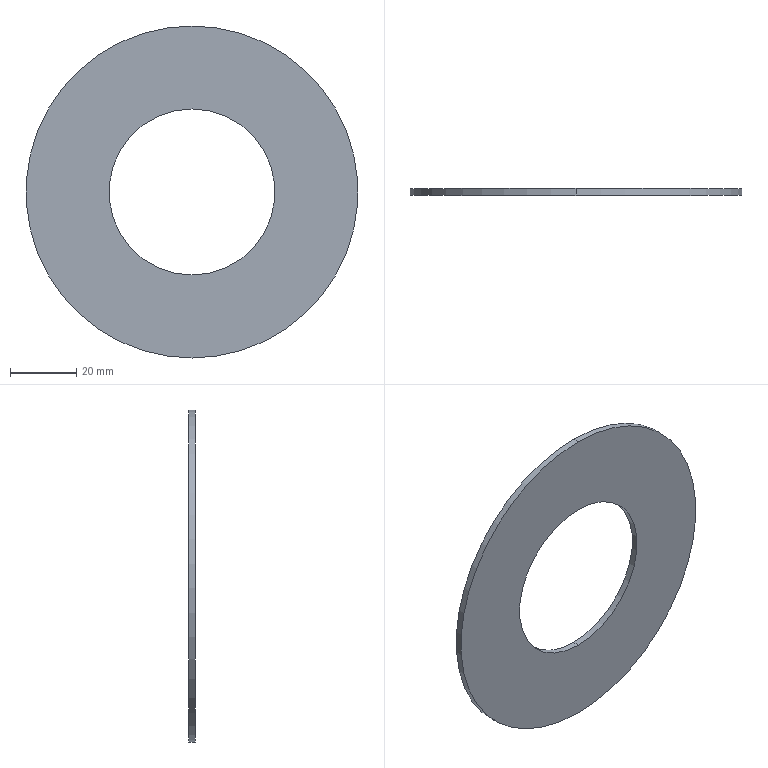Part | SolidWorks | features Extrusion 1 | 1 solid | 6 faces | box 100 x 2 x 100 mm | volume 11781 mm3 | cylinder 4 | plane 2 | commonest cylinder face diameters 50 x2 100 x2
STEP:
#1=CARTESIAN_POINT('',(0.,2.,-25.));
#2=VERTEX_POINT('',#1);
#3=CARTESIAN_POINT('',(0.,2.,25.));
#4=VERTEX_POINT('',#3);
#5=CARTESIAN_POINT('',(0.,2.,0.));
#6=DIRECTION('',(0.,1.,0.));
#7=DIRECTION('',(0.,0.,1.));
#8=AXIS2_PLACEMENT_3D('',#5,#6,#7);
#9=CIRCLE('',#8,25.);
#10=EDGE_CURVE('',#2,#4,#9,.T.);
#11=ORIENTED_EDGE('',*,*,#10,.T.);
#12=CARTESIAN_POINT('',(0.,0.,25.));
#13=VERTEX_POINT('',#12);
#14=CARTESIAN_POINT('',(0.,2.,25.));
#15=DIRECTION('',(0.,-1.,0.));
#16=VECTOR('',#15,1000.);
#17=LINE('',#14,#16);
#18=EDGE_CURVE('',#4,#13,#17,.T.);
#19=ORIENTED_EDGE('',*,*,#18,.T.);
#20=CARTESIAN_POINT('',(0.,0.,-25.));
#21=VERTEX_POINT('',#20);
#22=CARTESIAN_POINT('',(0.,0.,0.));
#23=DIRECTION('',(0.,1.,0.));
#24=DIRECTION('',(0.,0.,1.));
#25=AXIS2_PLACEMENT_3D('',#22,#23,#24);
#26=CIRCLE('',#25,25.);
#27=EDGE_CURVE('',#21,#13,#26,.T.);
#28=ORIENTED_EDGE('',*,*,#27,.F.);
#29=CARTESIAN_POINT('',(0.,2.,-25.));
#30=DIRECTION('',(0.,-1.,0.));
#31=VECTOR('',#30,1000.);
#32=LINE('',#29,#31);
#33=EDGE_CURVE('',#2,#21,#32,.T.);
#34=ORIENTED_EDGE('',*,*,#33,.F.);
#35=EDGE_LOOP('',(#11,#19,#28,#34));
#36=FACE_OUTER_BOUND('',#35,.T.);
#37=CARTESIAN_POINT('',(0.,2.,0.));
#38=DIRECTION('',(0.,-1.,0.));
#39=DIRECTION('',(0.,0.,-1.));
#40=AXIS2_PLACEMENT_3D('',#37,#38,#39);
#41=CYLINDRICAL_SURFACE('',#40,25.);
#42=ADVANCED_FACE('',(#36),#41,.F.);
#43=CARTESIAN_POINT('',(0.,2.,50.));
#44=VERTEX_POINT('',#43);
#45=CARTESIAN_POINT('',(0.,2.,-50.));
#46=VERTEX_POINT('',#45);
#47=CARTESIAN_POINT('',(0.,2.,0.));
#48=DIRECTION('',(0.,1.,0.));
#49=DIRECTION('',(0.,0.,1.));
#50=AXIS2_PLACEMENT_3D('',#47,#48,#49);
#51=CIRCLE('',#50,50.);
#52=EDGE_CURVE('',#44,#46,#51,.T.);
#53=ORIENTED_EDGE('',*,*,#52,.F.);
#54=CARTESIAN_POINT('',(0.,0.,50.));
#55=VERTEX_POINT('',#54);
#56=CARTESIAN_POINT('',(0.,2.,50.));
#57=DIRECTION('',(0.,-1.,0.));
#58=VECTOR('',#57,1000.);
#59=LINE('',#56,#58);
#60=EDGE_CURVE('',#44,#55,#59,.T.);
#61=ORIENTED_EDGE('',*,*,#60,.T.);
#62=CARTESIAN_POINT('',(0.,0.,-50.));
#63=VERTEX_POINT('',#62);
#64=CARTESIAN_POINT('',(0.,0.,0.));
#65=DIRECTION('',(0.,1.,0.));
#66=DIRECTION('',(0.,0.,1.));
#67=AXIS2_PLACEMENT_3D('',#64,#65,#66);
#68=CIRCLE('',#67,50.);
#69=EDGE_CURVE('',#55,#63,#68,.T.);
#70=ORIENTED_EDGE('',*,*,#69,.T.);
#71=CARTESIAN_POINT('',(0.,2.,-50.));
#72=DIRECTION('',(0.,-1.,0.));
#73=VECTOR('',#72,1000.);
#74=LINE('',#71,#73);
#75=EDGE_CURVE('',#46,#63,#74,.T.);
#76=ORIENTED_EDGE('',*,*,#75,.F.);
#77=EDGE_LOOP('',(#53,#61,#70,#76));
#78=FACE_OUTER_BOUND('',#77,.T.);
#79=CARTESIAN_POINT('',(0.,2.,0.));
#80=DIRECTION('',(0.,-1.,0.));
#81=DIRECTION('',(0.,0.,-1.));
#82=AXIS2_PLACEMENT_3D('',#79,#80,#81);
#83=CYLINDRICAL_SURFACE('',#82,50.);
#84=ADVANCED_FACE('',(#78),#83,.T.);
#85=CARTESIAN_POINT('',(0.,2.,0.));
#86=DIRECTION('',(0.,1.,0.));
#87=DIRECTION('',(0.,0.,1.));
#88=AXIS2_PLACEMENT_3D('',#85,#86,#87);
#89=CIRCLE('',#88,50.);
#90=EDGE_CURVE('',#46,#44,#89,.T.);
#91=ORIENTED_EDGE('',*,*,#90,.T.);
#92=ORIENTED_EDGE('',*,*,#52,.T.);
#93=EDGE_LOOP('',(#91,#92));
#94=FACE_OUTER_BOUND('',#93,.T.);
#95=ORIENTED_EDGE('',*,*,#10,.F.);
#96=CARTESIAN_POINT('',(0.,2.,0.));
#97=DIRECTION('',(0.,1.,0.));
#98=DIRECTION('',(0.,0.,1.));
#99=AXIS2_PLACEMENT_3D('',#96,#97,#98);
#100=CIRCLE('',#99,25.);
#101=EDGE_CURVE('',#4,#2,#100,.T.);
#102=ORIENTED_EDGE('',*,*,#101,.F.);
#103=EDGE_LOOP('',(#95,#102));
#104=FACE_BOUND('',#103,.T.);
#105=CARTESIAN_POINT('',(0.,2.,0.));
#106=DIRECTION('',(0.,1.,0.));
#107=DIRECTION('',(0.,0.,1.));
#108=AXIS2_PLACEMENT_3D('',#105,#106,#107);
#109=PLANE('',#108);
#110=ADVANCED_FACE('',(#94,#104),#109,.T.);
#111=CARTESIAN_POINT('',(0.,0.,0.));
#112=DIRECTION('',(0.,1.,0.));
#113=DIRECTION('',(0.,0.,1.));
#114=AXIS2_PLACEMENT_3D('',#111,#112,#113);
#115=CIRCLE('',#114,50.);
#116=EDGE_CURVE('',#63,#55,#115,.T.);
#117=ORIENTED_EDGE('',*,*,#116,.F.);
#118=ORIENTED_EDGE('',*,*,#69,.F.);
#119=EDGE_LOOP('',(#117,#118));
#120=FACE_OUTER_BOUND('',#119,.T.);
#121=ORIENTED_EDGE('',*,*,#27,.T.);
#122=CARTESIAN_POINT('',(0.,0.,0.));
#123=DIRECTION('',(0.,1.,0.));
#124=DIRECTION('',(0.,0.,1.));
#125=AXIS2_PLACEMENT_3D('',#122,#123,#124);
#126=CIRCLE('',#125,25.);
#127=EDGE_CURVE('',#13,#21,#126,.T.);
#128=ORIENTED_EDGE('',*,*,#127,.T.);
#129=EDGE_LOOP('',(#121,#128));
#130=FACE_BOUND('',#129,.T.);
#131=CARTESIAN_POINT('',(0.,0.,0.));
#132=DIRECTION('',(0.,1.,0.));
#133=DIRECTION('',(0.,0.,1.));
#134=AXIS2_PLACEMENT_3D('',#131,#132,#133);
#135=PLANE('',#134);
#136=ADVANCED_FACE('',(#120,#130),#135,.F.);
#137=ORIENTED_EDGE('',*,*,#60,.F.);
#138=ORIENTED_EDGE('',*,*,#90,.F.);
#139=ORIENTED_EDGE('',*,*,#75,.T.);
#140=ORIENTED_EDGE('',*,*,#116,.T.);
#141=EDGE_LOOP('',(#137,#138,#139,#140));
#142=FACE_OUTER_BOUND('',#141,.T.);
#143=CARTESIAN_POINT('',(0.,2.,0.));
#144=DIRECTION('',(0.,-1.,0.));
#145=DIRECTION('',(0.,0.,-1.));
#146=AXIS2_PLACEMENT_3D('',#143,#144,#145);
#147=CYLINDRICAL_SURFACE('',#146,50.);
#148=ADVANCED_FACE('',(#142),#147,.T.);
#149=ORIENTED_EDGE('',*,*,#18,.F.);
#150=ORIENTED_EDGE('',*,*,#101,.T.);
#151=ORIENTED_EDGE('',*,*,#33,.T.);
#152=ORIENTED_EDGE('',*,*,#127,.F.);
#153=EDGE_LOOP('',(#149,#150,#151,#152));
#154=FACE_OUTER_BOUND('',#153,.T.);
#155=CARTESIAN_POINT('',(0.,2.,0.));
#156=DIRECTION('',(0.,-1.,0.));
#157=DIRECTION('',(0.,0.,-1.));
#158=AXIS2_PLACEMENT_3D('',#155,#156,#157);
#159=CYLINDRICAL_SURFACE('',#158,25.);
#160=ADVANCED_FACE('',(#154),#159,.F.);
#161=CLOSED_SHELL('',(#42,#84,#110,#136,#148,#160));
#162=MANIFOLD_SOLID_BREP('',#161);
#163=CARTESIAN_POINT('',(0.,0.,0.));
#164=DIRECTION('',(0.,0.,1.));
#165=DIRECTION('',(1.,0.,0.));
#166=AXIS2_PLACEMENT_3D('',#163,#164,#165);
#167=(LENGTH_UNIT()NAMED_UNIT(*)SI_UNIT(.MILLI.,.METRE.));
#168=UNCERTAINTY_MEASURE_WITH_UNIT(LENGTH_MEASURE(0.00001),#167,'','');
#169=(NAMED_UNIT(*)PLANE_ANGLE_UNIT()SI_UNIT($,.RADIAN.));
#170=(NAMED_UNIT(*)SI_UNIT($,.STERADIAN.)SOLID_ANGLE_UNIT());
#171=(GEOMETRIC_REPRESENTATION_CONTEXT(3)GLOBAL_UNCERTAINTY_ASSIGNED_CONTEXT((#168))GLOBAL_UNIT_ASSIGNED_CONTEXT((#167,#169,#170))REPRESENTATION_CONTEXT('',''));
#172=ADVANCED_BREP_SHAPE_REPRESENTATION('',(#162,#166),#171);